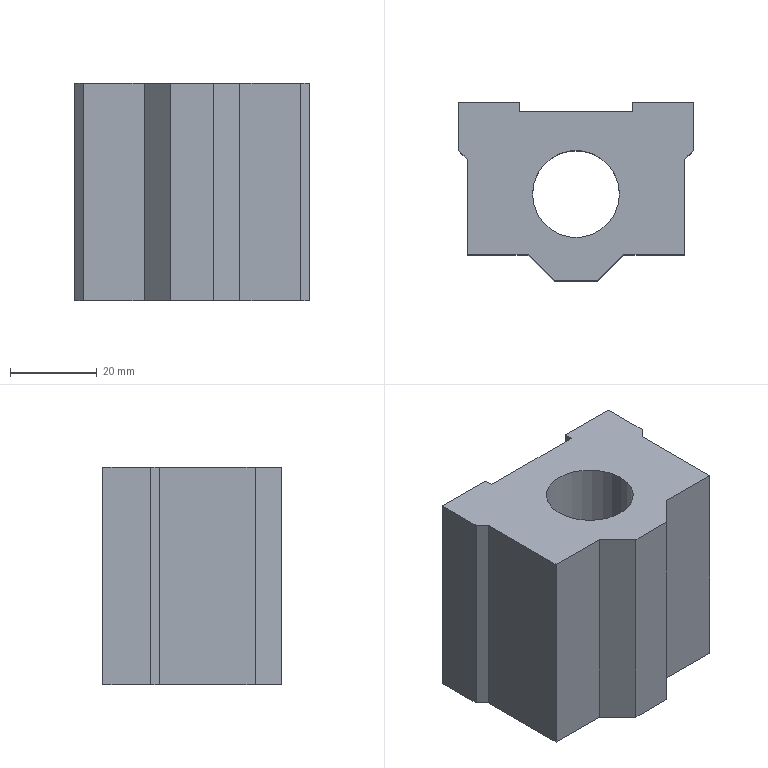Part | SolidWorks | features Extrusion 1, HoleWzd 1, LPattern 1 | 1 solid | 36 faces | box 54 x 41 x 50 mm | volume 75018 mm3 | plane 18 | cylinder 10 | cone 8 | commonest cylinder face diameters 5 x8 20 x2
STEP:
#1=CARTESIAN_POINT('',(-20.,2.498,45.));
#2=VERTEX_POINT('',#1);
#3=CARTESIAN_POINT('',(-20.,4.,47.5));
#4=VERTEX_POINT('',#3);
#5=CARTESIAN_POINT('',(-20.,4.,47.5));
#6=DIRECTION('',(0.,0.515,0.8572));
#7=VECTOR('',#6,1000.);
#8=LINE('',#5,#7);
#9=EDGE_CURVE('',#2,#4,#8,.T.);
#10=ORIENTED_EDGE('',*,*,#9,.F.);
#11=CARTESIAN_POINT('',(-20.,4.,42.5));
#12=VERTEX_POINT('',#11);
#13=CARTESIAN_POINT('',(-20.,4.,42.5));
#14=DIRECTION('',(0.,0.515,-0.8572));
#15=VECTOR('',#14,1000.);
#16=LINE('',#13,#15);
#17=EDGE_CURVE('',#2,#12,#16,.T.);
#18=ORIENTED_EDGE('',*,*,#17,.T.);
#19=CARTESIAN_POINT('',(-20.,4.,45.));
#20=DIRECTION('',(0.,1.,0.));
#21=DIRECTION('',(0.,0.,1.));
#22=AXIS2_PLACEMENT_3D('',#19,#20,#21);
#23=CIRCLE('',#22,2.5);
#24=EDGE_CURVE('',#12,#4,#23,.T.);
#25=ORIENTED_EDGE('',*,*,#24,.T.);
#26=EDGE_LOOP('',(#10,#18,#25));
#27=FACE_OUTER_BOUND('',#26,.T.);
#28=CARTESIAN_POINT('',(-20.,4.,45.));
#29=DIRECTION('',(0.,1.,0.));
#30=DIRECTION('',(0.,0.,1.));
#31=AXIS2_PLACEMENT_3D('',#28,#29,#30);
#32=CONICAL_SURFACE('',#31,2.5,1.03);
#33=ADVANCED_FACE('',(#27),#32,.F.);
#34=ORIENTED_EDGE('',*,*,#24,.F.);
#35=CARTESIAN_POINT('',(-20.,21.,42.5));
#36=VERTEX_POINT('',#35);
#37=CARTESIAN_POINT('',(-20.,21.,42.5));
#38=DIRECTION('',(0.,1.,0.));
#39=VECTOR('',#38,1000.);
#40=LINE('',#37,#39);
#41=EDGE_CURVE('',#12,#36,#40,.T.);
#42=ORIENTED_EDGE('',*,*,#41,.T.);
#43=CARTESIAN_POINT('',(-20.,21.,47.5));
#44=VERTEX_POINT('',#43);
#45=CARTESIAN_POINT('',(-20.,21.,45.));
#46=DIRECTION('',(0.,1.,0.));
#47=DIRECTION('',(0.,0.,1.));
#48=AXIS2_PLACEMENT_3D('',#45,#46,#47);
#49=CIRCLE('',#48,2.5);
#50=EDGE_CURVE('',#36,#44,#49,.T.);
#51=ORIENTED_EDGE('',*,*,#50,.T.);
#52=CARTESIAN_POINT('',(-20.,21.,47.5));
#53=DIRECTION('',(0.,1.,0.));
#54=VECTOR('',#53,1000.);
#55=LINE('',#52,#54);
#56=EDGE_CURVE('',#4,#44,#55,.T.);
#57=ORIENTED_EDGE('',*,*,#56,.F.);
#58=EDGE_LOOP('',(#34,#42,#51,#57));
#59=FACE_OUTER_BOUND('',#58,.T.);
#60=CARTESIAN_POINT('',(-20.,21.,45.));
#61=DIRECTION('',(0.,1.,0.));
#62=DIRECTION('',(0.,0.,1.));
#63=AXIS2_PLACEMENT_3D('',#60,#61,#62);
#64=CYLINDRICAL_SURFACE('',#63,2.5);
#65=ADVANCED_FACE('',(#59),#64,.F.);
#66=CARTESIAN_POINT('',(20.,2.498,45.));
#67=VERTEX_POINT('',#66);
#68=CARTESIAN_POINT('',(20.,4.,47.5));
#69=VERTEX_POINT('',#68);
#70=CARTESIAN_POINT('',(20.,4.,47.5));
#71=DIRECTION('',(0.,0.515,0.8572));
#72=VECTOR('',#71,1000.);
#73=LINE('',#70,#72);
#74=EDGE_CURVE('',#67,#69,#73,.T.);
#75=ORIENTED_EDGE('',*,*,#74,.F.);
#76=CARTESIAN_POINT('',(20.,4.,42.5));
#77=VERTEX_POINT('',#76);
#78=CARTESIAN_POINT('',(20.,4.,42.5));
#79=DIRECTION('',(0.,0.515,-0.8572));
#80=VECTOR('',#79,1000.);
#81=LINE('',#78,#80);
#82=EDGE_CURVE('',#67,#77,#81,.T.);
#83=ORIENTED_EDGE('',*,*,#82,.T.);
#84=CARTESIAN_POINT('',(20.,4.,45.));
#85=DIRECTION('',(0.,1.,0.));
#86=DIRECTION('',(0.,0.,1.));
#87=AXIS2_PLACEMENT_3D('',#84,#85,#86);
#88=CIRCLE('',#87,2.5);
#89=EDGE_CURVE('',#77,#69,#88,.T.);
#90=ORIENTED_EDGE('',*,*,#89,.T.);
#91=EDGE_LOOP('',(#75,#83,#90));
#92=FACE_OUTER_BOUND('',#91,.T.);
#93=CARTESIAN_POINT('',(20.,4.,45.));
#94=DIRECTION('',(0.,1.,0.));
#95=DIRECTION('',(0.,0.,1.));
#96=AXIS2_PLACEMENT_3D('',#93,#94,#95);
#97=CONICAL_SURFACE('',#96,2.5,1.03);
#98=ADVANCED_FACE('',(#92),#97,.F.);
#99=ORIENTED_EDGE('',*,*,#89,.F.);
#100=CARTESIAN_POINT('',(20.,21.,42.5));
#101=VERTEX_POINT('',#100);
#102=CARTESIAN_POINT('',(20.,21.,42.5));
#103=DIRECTION('',(0.,1.,0.));
#104=VECTOR('',#103,1000.);
#105=LINE('',#102,#104);
#106=EDGE_CURVE('',#77,#101,#105,.T.);
#107=ORIENTED_EDGE('',*,*,#106,.T.);
#108=CARTESIAN_POINT('',(20.,21.,47.5));
#109=VERTEX_POINT('',#108);
#110=CARTESIAN_POINT('',(20.,21.,45.));
#111=DIRECTION('',(0.,1.,0.));
#112=DIRECTION('',(0.,0.,1.));
#113=AXIS2_PLACEMENT_3D('',#110,#111,#112);
#114=CIRCLE('',#113,2.5);
#115=EDGE_CURVE('',#101,#109,#114,.T.);
#116=ORIENTED_EDGE('',*,*,#115,.T.);
#117=CARTESIAN_POINT('',(20.,21.,47.5));
#118=DIRECTION('',(0.,1.,0.));
#119=VECTOR('',#118,1000.);
#120=LINE('',#117,#119);
#121=EDGE_CURVE('',#69,#109,#120,.T.);
#122=ORIENTED_EDGE('',*,*,#121,.F.);
#123=EDGE_LOOP('',(#99,#107,#116,#122));
#124=FACE_OUTER_BOUND('',#123,.T.);
#125=CARTESIAN_POINT('',(20.,21.,45.));
#126=DIRECTION('',(0.,1.,0.));
#127=DIRECTION('',(0.,0.,1.));
#128=AXIS2_PLACEMENT_3D('',#125,#126,#127);
#129=CYLINDRICAL_SURFACE('',#128,2.5);
#130=ADVANCED_FACE('',(#124),#129,.F.);
#131=CARTESIAN_POINT('',(-20.,2.498,5.));
#132=VERTEX_POINT('',#131);
#133=CARTESIAN_POINT('',(-20.,4.,7.5));
#134=VERTEX_POINT('',#133);
#135=CARTESIAN_POINT('',(-20.,4.,7.5));
#136=DIRECTION('',(0.,0.515,0.8572));
#137=VECTOR('',#136,1000.);
#138=LINE('',#135,#137);
#139=EDGE_CURVE('',#132,#134,#138,.T.);
#140=ORIENTED_EDGE('',*,*,#139,.F.);
#141=CARTESIAN_POINT('',(-20.,4.,2.5));
#142=VERTEX_POINT('',#141);
#143=CARTESIAN_POINT('',(-20.,4.,2.5));
#144=DIRECTION('',(0.,0.515,-0.8572));
#145=VECTOR('',#144,1000.);
#146=LINE('',#143,#145);
#147=EDGE_CURVE('',#132,#142,#146,.T.);
#148=ORIENTED_EDGE('',*,*,#147,.T.);
#149=CARTESIAN_POINT('',(-20.,4.,5.));
#150=DIRECTION('',(0.,1.,0.));
#151=DIRECTION('',(0.,0.,1.));
#152=AXIS2_PLACEMENT_3D('',#149,#150,#151);
#153=CIRCLE('',#152,2.5);
#154=EDGE_CURVE('',#142,#134,#153,.T.);
#155=ORIENTED_EDGE('',*,*,#154,.T.);
#156=EDGE_LOOP('',(#140,#148,#155));
#157=FACE_OUTER_BOUND('',#156,.T.);
#158=CARTESIAN_POINT('',(-20.,4.,5.));
#159=DIRECTION('',(0.,1.,0.));
#160=DIRECTION('',(0.,0.,1.));
#161=AXIS2_PLACEMENT_3D('',#158,#159,#160);
#162=CONICAL_SURFACE('',#161,2.5,1.03);
#163=ADVANCED_FACE('',(#157),#162,.F.);
#164=ORIENTED_EDGE('',*,*,#154,.F.);
#165=CARTESIAN_POINT('',(-20.,21.,2.5));
#166=VERTEX_POINT('',#165);
#167=CARTESIAN_POINT('',(-20.,21.,2.5));
#168=DIRECTION('',(0.,1.,0.));
#169=VECTOR('',#168,1000.);
#170=LINE('',#167,#169);
#171=EDGE_CURVE('',#142,#166,#170,.T.);
#172=ORIENTED_EDGE('',*,*,#171,.T.);
#173=CARTESIAN_POINT('',(-20.,21.,7.5));
#174=VERTEX_POINT('',#173);
#175=CARTESIAN_POINT('',(-20.,21.,5.));
#176=DIRECTION('',(0.,1.,0.));
#177=DIRECTION('',(0.,0.,1.));
#178=AXIS2_PLACEMENT_3D('',#175,#176,#177);
#179=CIRCLE('',#178,2.5);
#180=EDGE_CURVE('',#166,#174,#179,.T.);
#181=ORIENTED_EDGE('',*,*,#180,.T.);
#182=CARTESIAN_POINT('',(-20.,21.,7.5));
#183=DIRECTION('',(0.,1.,0.));
#184=VECTOR('',#183,1000.);
#185=LINE('',#182,#184);
#186=EDGE_CURVE('',#134,#174,#185,.T.);
#187=ORIENTED_EDGE('',*,*,#186,.F.);
#188=EDGE_LOOP('',(#164,#172,#181,#187));
#189=FACE_OUTER_BOUND('',#188,.T.);
#190=CARTESIAN_POINT('',(-20.,21.,5.));
#191=DIRECTION('',(0.,1.,0.));
#192=DIRECTION('',(0.,0.,1.));
#193=AXIS2_PLACEMENT_3D('',#190,#191,#192);
#194=CYLINDRICAL_SURFACE('',#193,2.5);
#195=ADVANCED_FACE('',(#189),#194,.F.);
#196=CARTESIAN_POINT('',(20.,2.498,5.));
#197=VERTEX_POINT('',#196);
#198=CARTESIAN_POINT('',(20.,4.,7.5));
#199=VERTEX_POINT('',#198);
#200=CARTESIAN_POINT('',(20.,4.,7.5));
#201=DIRECTION('',(0.,0.515,0.8572));
#202=VECTOR('',#201,1000.);
#203=LINE('',#200,#202);
#204=EDGE_CURVE('',#197,#199,#203,.T.);
#205=ORIENTED_EDGE('',*,*,#204,.F.);
#206=CARTESIAN_POINT('',(20.,4.,2.5));
#207=VERTEX_POINT('',#206);
#208=CARTESIAN_POINT('',(20.,4.,2.5));
#209=DIRECTION('',(0.,0.515,-0.8572));
#210=VECTOR('',#209,1000.);
#211=LINE('',#208,#210);
#212=EDGE_CURVE('',#197,#207,#211,.T.);
#213=ORIENTED_EDGE('',*,*,#212,.T.);
#214=CARTESIAN_POINT('',(20.,4.,5.));
#215=DIRECTION('',(0.,1.,0.));
#216=DIRECTION('',(0.,0.,1.));
#217=AXIS2_PLACEMENT_3D('',#214,#215,#216);
#218=CIRCLE('',#217,2.5);
#219=EDGE_CURVE('',#207,#199,#218,.T.);
#220=ORIENTED_EDGE('',*,*,#219,.T.);
#221=EDGE_LOOP('',(#205,#213,#220));
#222=FACE_OUTER_BOUND('',#221,.T.);
#223=CARTESIAN_POINT('',(20.,4.,5.));
#224=DIRECTION('',(0.,1.,0.));
#225=DIRECTION('',(0.,0.,1.));
#226=AXIS2_PLACEMENT_3D('',#223,#224,#225);
#227=CONICAL_SURFACE('',#226,2.5,1.03);
#228=ADVANCED_FACE('',(#222),#227,.F.);
#229=ORIENTED_EDGE('',*,*,#219,.F.);
#230=CARTESIAN_POINT('',(20.,21.,2.5));
#231=VERTEX_POINT('',#230);
#232=CARTESIAN_POINT('',(20.,21.,2.5));
#233=DIRECTION('',(0.,1.,0.));
#234=VECTOR('',#233,1000.);
#235=LINE('',#232,#234);
#236=EDGE_CURVE('',#207,#231,#235,.T.);
#237=ORIENTED_EDGE('',*,*,#236,.T.);
#238=CARTESIAN_POINT('',(20.,21.,7.5));
#239=VERTEX_POINT('',#238);
#240=CARTESIAN_POINT('',(20.,21.,5.));
#241=DIRECTION('',(0.,1.,0.));
#242=DIRECTION('',(0.,0.,1.));
#243=AXIS2_PLACEMENT_3D('',#240,#241,#242);
#244=CIRCLE('',#243,2.5);
#245=EDGE_CURVE('',#231,#239,#244,.T.);
#246=ORIENTED_EDGE('',*,*,#245,.T.);
#247=CARTESIAN_POINT('',(20.,21.,7.5));
#248=DIRECTION('',(0.,1.,0.));
#249=VECTOR('',#248,1000.);
#250=LINE('',#247,#249);
#251=EDGE_CURVE('',#199,#239,#250,.T.);
#252=ORIENTED_EDGE('',*,*,#251,.F.);
#253=EDGE_LOOP('',(#229,#237,#246,#252));
#254=FACE_OUTER_BOUND('',#253,.T.);
#255=CARTESIAN_POINT('',(20.,21.,5.));
#256=DIRECTION('',(0.,1.,0.));
#257=DIRECTION('',(0.,0.,1.));
#258=AXIS2_PLACEMENT_3D('',#255,#256,#257);
#259=CYLINDRICAL_SURFACE('',#258,2.5);
#260=ADVANCED_FACE('',(#254),#259,.F.);
#261=CARTESIAN_POINT('',(-10.,0.,50.));
#262=VERTEX_POINT('',#261);
#263=CARTESIAN_POINT('',(10.,0.,50.));
#264=VERTEX_POINT('',#263);
#265=CARTESIAN_POINT('',(0.,0.,50.));
#266=DIRECTION('',(0.,0.,1.));
#267=DIRECTION('',(1.,0.,0.));
#268=AXIS2_PLACEMENT_3D('',#265,#266,#267);
#269=CIRCLE('',#268,10.);
#270=EDGE_CURVE('',#262,#264,#269,.T.);
#271=ORIENTED_EDGE('',*,*,#270,.T.);
#272=CARTESIAN_POINT('',(10.,0.,0.));
#273=VERTEX_POINT('',#272);
#274=CARTESIAN_POINT('',(10.,0.,50.));
#275=DIRECTION('',(0.,0.,-1.));
#276=VECTOR('',#275,1000.);
#277=LINE('',#274,#276);
#278=EDGE_CURVE('',#264,#273,#277,.T.);
#279=ORIENTED_EDGE('',*,*,#278,.T.);
#280=CARTESIAN_POINT('',(-10.,0.,0.));
#281=VERTEX_POINT('',#280);
#282=CARTESIAN_POINT('',(0.,0.,0.));
#283=DIRECTION('',(0.,0.,1.));
#284=DIRECTION('',(1.,0.,0.));
#285=AXIS2_PLACEMENT_3D('',#282,#283,#284);
#286=CIRCLE('',#285,10.);
#287=EDGE_CURVE('',#281,#273,#286,.T.);
#288=ORIENTED_EDGE('',*,*,#287,.F.);
#289=CARTESIAN_POINT('',(-10.,0.,50.));
#290=DIRECTION('',(0.,0.,-1.));
#291=VECTOR('',#290,1000.);
#292=LINE('',#289,#291);
#293=EDGE_CURVE('',#262,#281,#292,.T.);
#294=ORIENTED_EDGE('',*,*,#293,.F.);
#295=EDGE_LOOP('',(#271,#279,#288,#294));
#296=FACE_OUTER_BOUND('',#295,.T.);
#297=CARTESIAN_POINT('',(0.,0.,50.));
#298=DIRECTION('',(0.,0.,-1.));
#299=DIRECTION('',(-1.,0.,0.));
#300=AXIS2_PLACEMENT_3D('',#297,#298,#299);
#301=CYLINDRICAL_SURFACE('',#300,10.);
#302=ADVANCED_FACE('',(#296),#301,.F.);
#303=CARTESIAN_POINT('',(-11.,-14.,50.));
#304=VERTEX_POINT('',#303);
#305=CARTESIAN_POINT('',(-5.,-20.,50.));
#306=VERTEX_POINT('',#305);
#307=CARTESIAN_POINT('',(-5.,-20.,50.));
#308=DIRECTION('',(0.7071,-0.7071,0.));
#309=VECTOR('',#308,1000.);
#310=LINE('',#307,#309);
#311=EDGE_CURVE('',#304,#306,#310,.T.);
#312=ORIENTED_EDGE('',*,*,#311,.T.);
#313=CARTESIAN_POINT('',(5.,-20.,50.));
#314=VERTEX_POINT('',#313);
#315=CARTESIAN_POINT('',(5.,-20.,50.));
#316=DIRECTION('',(1.,0.,0.));
#317=VECTOR('',#316,1000.);
#318=LINE('',#315,#317);
#319=EDGE_CURVE('',#306,#314,#318,.T.);
#320=ORIENTED_EDGE('',*,*,#319,.T.);
#321=CARTESIAN_POINT('',(11.,-14.,50.));
#322=VERTEX_POINT('',#321);
#323=CARTESIAN_POINT('',(5.,-20.,50.));
#324=DIRECTION('',(0.7071,0.7071,0.));
#325=VECTOR('',#324,1000.);
#326=LINE('',#323,#325);
#327=EDGE_CURVE('',#314,#322,#326,.T.);
#328=ORIENTED_EDGE('',*,*,#327,.T.);
#329=CARTESIAN_POINT('',(25.,-14.,50.));
#330=VERTEX_POINT('',#329);
#331=CARTESIAN_POINT('',(11.,-14.,50.));
#332=DIRECTION('',(1.,0.,0.));
#333=VECTOR('',#332,1000.);
#334=LINE('',#331,#333);
#335=EDGE_CURVE('',#322,#330,#334,.T.);
#336=ORIENTED_EDGE('',*,*,#335,.T.);
#337=CARTESIAN_POINT('',(25.,8.,50.));
#338=VERTEX_POINT('',#337);
#339=CARTESIAN_POINT('',(25.,-14.,50.));
#340=DIRECTION('',(0.,1.,0.));
#341=VECTOR('',#340,1000.);
#342=LINE('',#339,#341);
#343=EDGE_CURVE('',#330,#338,#342,.T.);
#344=ORIENTED_EDGE('',*,*,#343,.T.);
#345=CARTESIAN_POINT('',(27.,10.,50.));
#346=VERTEX_POINT('',#345);
#347=CARTESIAN_POINT('',(25.,8.,50.));
#348=DIRECTION('',(0.7071,0.7071,0.));
#349=VECTOR('',#348,1000.);
#350=LINE('',#347,#349);
#351=EDGE_CURVE('',#338,#346,#350,.T.);
#352=ORIENTED_EDGE('',*,*,#351,.T.);
#353=CARTESIAN_POINT('',(27.,21.,50.));
#354=VERTEX_POINT('',#353);
#355=CARTESIAN_POINT('',(27.,10.,50.));
#356=DIRECTION('',(0.,1.,0.));
#357=VECTOR('',#356,1000.);
#358=LINE('',#355,#357);
#359=EDGE_CURVE('',#346,#354,#358,.T.);
#360=ORIENTED_EDGE('',*,*,#359,.T.);
#361=CARTESIAN_POINT('',(13.,21.,50.));
#362=VERTEX_POINT('',#361);
#363=CARTESIAN_POINT('',(27.,21.,50.));
#364=DIRECTION('',(-1.,0.,0.));
#365=VECTOR('',#364,1000.);
#366=LINE('',#363,#365);
#367=EDGE_CURVE('',#354,#362,#366,.T.);
#368=ORIENTED_EDGE('',*,*,#367,.T.);
#369=CARTESIAN_POINT('',(13.,19.,50.));
#370=VERTEX_POINT('',#369);
#371=CARTESIAN_POINT('',(13.,21.,50.));
#372=DIRECTION('',(0.,-1.,0.));
#373=VECTOR('',#372,1000.);
#374=LINE('',#371,#373);
#375=EDGE_CURVE('',#362,#370,#374,.T.);
#376=ORIENTED_EDGE('',*,*,#375,.T.);
#377=CARTESIAN_POINT('',(-13.,19.,50.));
#378=VERTEX_POINT('',#377);
#379=CARTESIAN_POINT('',(-13.,19.,50.));
#380=DIRECTION('',(-1.,0.,0.));
#381=VECTOR('',#380,1000.);
#382=LINE('',#379,#381);
#383=EDGE_CURVE('',#370,#378,#382,.T.);
#384=ORIENTED_EDGE('',*,*,#383,.T.);
#385=CARTESIAN_POINT('',(-13.,21.,50.));
#386=VERTEX_POINT('',#385);
#387=CARTESIAN_POINT('',(-13.,21.,50.));
#388=DIRECTION('',(0.,1.,0.));
#389=VECTOR('',#388,1000.);
#390=LINE('',#387,#389);
#391=EDGE_CURVE('',#378,#386,#390,.T.);
#392=ORIENTED_EDGE('',*,*,#391,.T.);
#393=CARTESIAN_POINT('',(-27.,21.,50.));
#394=VERTEX_POINT('',#393);
#395=CARTESIAN_POINT('',(-27.,21.,50.));
#396=DIRECTION('',(-1.,0.,0.));
#397=VECTOR('',#396,1000.);
#398=LINE('',#395,#397);
#399=EDGE_CURVE('',#386,#394,#398,.T.);
#400=ORIENTED_EDGE('',*,*,#399,.T.);
#401=CARTESIAN_POINT('',(-27.,10.,50.));
#402=VERTEX_POINT('',#401);
#403=CARTESIAN_POINT('',(-27.,10.,50.));
#404=DIRECTION('',(0.,-1.,0.));
#405=VECTOR('',#404,1000.);
#406=LINE('',#403,#405);
#407=EDGE_CURVE('',#394,#402,#406,.T.);
#408=ORIENTED_EDGE('',*,*,#407,.T.);
#409=CARTESIAN_POINT('',(-25.,8.,50.));
#410=VERTEX_POINT('',#409);
#411=CARTESIAN_POINT('',(-25.,8.,50.));
#412=DIRECTION('',(0.7071,-0.7071,0.));
#413=VECTOR('',#412,1000.);
#414=LINE('',#411,#413);
#415=EDGE_CURVE('',#402,#410,#414,.T.);
#416=ORIENTED_EDGE('',*,*,#415,.T.);
#417=CARTESIAN_POINT('',(-25.,-14.,50.));
#418=VERTEX_POINT('',#417);
#419=CARTESIAN_POINT('',(-25.,-14.,50.));
#420=DIRECTION('',(0.,-1.,0.));
#421=VECTOR('',#420,1000.);
#422=LINE('',#419,#421);
#423=EDGE_CURVE('',#410,#418,#422,.T.);
#424=ORIENTED_EDGE('',*,*,#423,.T.);
#425=CARTESIAN_POINT('',(-11.,-14.,50.));
#426=DIRECTION('',(1.,0.,0.));
#427=VECTOR('',#426,1000.);
#428=LINE('',#425,#427);
#429=EDGE_CURVE('',#418,#304,#428,.T.);
#430=ORIENTED_EDGE('',*,*,#429,.T.);
#431=EDGE_LOOP('',(#312,#320,#328,#336,#344,#352,#360,#368,#376,#384,#392,#400,#408,#416,#424,#430));
#432=FACE_OUTER_BOUND('',#431,.T.);
#433=ORIENTED_EDGE('',*,*,#270,.F.);
#434=CARTESIAN_POINT('',(0.,0.,50.));
#435=DIRECTION('',(0.,0.,1.));
#436=DIRECTION('',(1.,0.,0.));
#437=AXIS2_PLACEMENT_3D('',#434,#435,#436);
#438=CIRCLE('',#437,10.);
#439=EDGE_CURVE('',#264,#262,#438,.T.);
#440=ORIENTED_EDGE('',*,*,#439,.F.);
#441=EDGE_LOOP('',(#433,#440));
#442=FACE_BOUND('',#441,.T.);
#443=CARTESIAN_POINT('',(-4.,-21.,50.));
#444=DIRECTION('',(0.,0.,-1.));
#445=DIRECTION('',(-1.,0.,0.));
#446=AXIS2_PLACEMENT_3D('',#443,#444,#445);
#447=PLANE('',#446);
#448=ADVANCED_FACE('',(#432,#442),#447,.F.);
#449=CARTESIAN_POINT('',(-11.,-14.,0.));
#450=VERTEX_POINT('',#449);
#451=CARTESIAN_POINT('',(-5.,-20.,0.));
#452=VERTEX_POINT('',#451);
#453=CARTESIAN_POINT('',(-5.,-20.,0.));
#454=DIRECTION('',(0.7071,-0.7071,0.));
#455=VECTOR('',#454,1000.);
#456=LINE('',#453,#455);
#457=EDGE_CURVE('',#450,#452,#456,.T.);
#458=ORIENTED_EDGE('',*,*,#457,.F.);
#459=CARTESIAN_POINT('',(-25.,-14.,0.));
#460=VERTEX_POINT('',#459);
#461=CARTESIAN_POINT('',(-11.,-14.,0.));
#462=DIRECTION('',(1.,0.,0.));
#463=VECTOR('',#462,1000.);
#464=LINE('',#461,#463);
#465=EDGE_CURVE('',#460,#450,#464,.T.);
#466=ORIENTED_EDGE('',*,*,#465,.F.);
#467=CARTESIAN_POINT('',(-25.,8.,0.));
#468=VERTEX_POINT('',#467);
#469=CARTESIAN_POINT('',(-25.,-14.,0.));
#470=DIRECTION('',(0.,-1.,0.));
#471=VECTOR('',#470,1000.);
#472=LINE('',#469,#471);
#473=EDGE_CURVE('',#468,#460,#472,.T.);
#474=ORIENTED_EDGE('',*,*,#473,.F.);
#475=CARTESIAN_POINT('',(-27.,10.,0.));
#476=VERTEX_POINT('',#475);
#477=CARTESIAN_POINT('',(-25.,8.,0.));
#478=DIRECTION('',(0.7071,-0.7071,0.));
#479=VECTOR('',#478,1000.);
#480=LINE('',#477,#479);
#481=EDGE_CURVE('',#476,#468,#480,.T.);
#482=ORIENTED_EDGE('',*,*,#481,.F.);
#483=CARTESIAN_POINT('',(-27.,21.,0.));
#484=VERTEX_POINT('',#483);
#485=CARTESIAN_POINT('',(-27.,10.,0.));
#486=DIRECTION('',(0.,-1.,0.));
#487=VECTOR('',#486,1000.);
#488=LINE('',#485,#487);
#489=EDGE_CURVE('',#484,#476,#488,.T.);
#490=ORIENTED_EDGE('',*,*,#489,.F.);
#491=CARTESIAN_POINT('',(-13.,21.,0.));
#492=VERTEX_POINT('',#491);
#493=CARTESIAN_POINT('',(-27.,21.,0.));
#494=DIRECTION('',(-1.,0.,0.));
#495=VECTOR('',#494,1000.);
#496=LINE('',#493,#495);
#497=EDGE_CURVE('',#492,#484,#496,.T.);
#498=ORIENTED_EDGE('',*,*,#497,.F.);
#499=CARTESIAN_POINT('',(-13.,19.,0.));
#500=VERTEX_POINT('',#499);
#501=CARTESIAN_POINT('',(-13.,21.,0.));
#502=DIRECTION('',(0.,1.,0.));
#503=VECTOR('',#502,1000.);
#504=LINE('',#501,#503);
#505=EDGE_CURVE('',#500,#492,#504,.T.);
#506=ORIENTED_EDGE('',*,*,#505,.F.);
#507=CARTESIAN_POINT('',(13.,19.,0.));
#508=VERTEX_POINT('',#507);
#509=CARTESIAN_POINT('',(-13.,19.,0.));
#510=DIRECTION('',(-1.,0.,0.));
#511=VECTOR('',#510,1000.);
#512=LINE('',#509,#511);
#513=EDGE_CURVE('',#508,#500,#512,.T.);
#514=ORIENTED_EDGE('',*,*,#513,.F.);
#515=CARTESIAN_POINT('',(13.,21.,0.));
#516=VERTEX_POINT('',#515);
#517=CARTESIAN_POINT('',(13.,21.,0.));
#518=DIRECTION('',(0.,-1.,0.));
#519=VECTOR('',#518,1000.);
#520=LINE('',#517,#519);
#521=EDGE_CURVE('',#516,#508,#520,.T.);
#522=ORIENTED_EDGE('',*,*,#521,.F.);
#523=CARTESIAN_POINT('',(27.,21.,0.));
#524=VERTEX_POINT('',#523);
#525=CARTESIAN_POINT('',(27.,21.,0.));
#526=DIRECTION('',(-1.,0.,0.));
#527=VECTOR('',#526,1000.);
#528=LINE('',#525,#527);
#529=EDGE_CURVE('',#524,#516,#528,.T.);
#530=ORIENTED_EDGE('',*,*,#529,.F.);
#531=CARTESIAN_POINT('',(27.,10.,0.));
#532=VERTEX_POINT('',#531);
#533=CARTESIAN_POINT('',(27.,10.,0.));
#534=DIRECTION('',(0.,1.,0.));
#535=VECTOR('',#534,1000.);
#536=LINE('',#533,#535);
#537=EDGE_CURVE('',#532,#524,#536,.T.);
#538=ORIENTED_EDGE('',*,*,#537,.F.);
#539=CARTESIAN_POINT('',(25.,8.,0.));
#540=VERTEX_POINT('',#539);
#541=CARTESIAN_POINT('',(25.,8.,0.));
#542=DIRECTION('',(0.7071,0.7071,0.));
#543=VECTOR('',#542,1000.);
#544=LINE('',#541,#543);
#545=EDGE_CURVE('',#540,#532,#544,.T.);
#546=ORIENTED_EDGE('',*,*,#545,.F.);
#547=CARTESIAN_POINT('',(25.,-14.,0.));
#548=VERTEX_POINT('',#547);
#549=CARTESIAN_POINT('',(25.,-14.,0.));
#550=DIRECTION('',(0.,1.,0.));
#551=VECTOR('',#550,1000.);
#552=LINE('',#549,#551);
#553=EDGE_CURVE('',#548,#540,#552,.T.);
#554=ORIENTED_EDGE('',*,*,#553,.F.);
#555=CARTESIAN_POINT('',(11.,-14.,0.));
#556=VERTEX_POINT('',#555);
#557=CARTESIAN_POINT('',(11.,-14.,0.));
#558=DIRECTION('',(1.,0.,0.));
#559=VECTOR('',#558,1000.);
#560=LINE('',#557,#559);
#561=EDGE_CURVE('',#556,#548,#560,.T.);
#562=ORIENTED_EDGE('',*,*,#561,.F.);
#563=CARTESIAN_POINT('',(5.,-20.,0.));
#564=VERTEX_POINT('',#563);
#565=CARTESIAN_POINT('',(5.,-20.,0.));
#566=DIRECTION('',(0.7071,0.7071,0.));
#567=VECTOR('',#566,1000.);
#568=LINE('',#565,#567);
#569=EDGE_CURVE('',#564,#556,#568,.T.);
#570=ORIENTED_EDGE('',*,*,#569,.F.);
#571=CARTESIAN_POINT('',(5.,-20.,0.));
#572=DIRECTION('',(1.,0.,0.));
#573=VECTOR('',#572,1000.);
#574=LINE('',#571,#573);
#575=EDGE_CURVE('',#452,#564,#574,.T.);
#576=ORIENTED_EDGE('',*,*,#575,.F.);
#577=EDGE_LOOP('',(#458,#466,#474,#482,#490,#498,#506,#514,#522,#530,#538,#546,#554,#562,#570,#576));
#578=FACE_OUTER_BOUND('',#577,.T.);
#579=ORIENTED_EDGE('',*,*,#287,.T.);
#580=CARTESIAN_POINT('',(0.,0.,0.));
#581=DIRECTION('',(0.,0.,1.));
#582=DIRECTION('',(1.,0.,0.));
#583=AXIS2_PLACEMENT_3D('',#580,#581,#582);
#584=CIRCLE('',#583,10.);
#585=EDGE_CURVE('',#273,#281,#584,.T.);
#586=ORIENTED_EDGE('',*,*,#585,.T.);
#587=EDGE_LOOP('',(#579,#586));
#588=FACE_BOUND('',#587,.T.);
#589=CARTESIAN_POINT('',(-4.,-21.,0.));
#590=DIRECTION('',(0.,0.,-1.));
#591=DIRECTION('',(-1.,0.,0.));
#592=AXIS2_PLACEMENT_3D('',#589,#590,#591);
#593=PLANE('',#592);
#594=ADVANCED_FACE('',(#578,#588),#593,.T.);
#595=ORIENTED_EDGE('',*,*,#457,.T.);
#596=CARTESIAN_POINT('',(-5.,-20.,50.));
#597=DIRECTION('',(0.,0.,-1.));
#598=VECTOR('',#597,1000.);
#599=LINE('',#596,#598);
#600=EDGE_CURVE('',#306,#452,#599,.T.);
#601=ORIENTED_EDGE('',*,*,#600,.F.);
#602=ORIENTED_EDGE('',*,*,#311,.F.);
#603=CARTESIAN_POINT('',(-11.,-14.,50.));
#604=DIRECTION('',(0.,0.,-1.));
#605=VECTOR('',#604,1000.);
#606=LINE('',#603,#605);
#607=EDGE_CURVE('',#304,#450,#606,.T.);
#608=ORIENTED_EDGE('',*,*,#607,.T.);
#609=EDGE_LOOP('',(#595,#601,#602,#608));
#610=FACE_OUTER_BOUND('',#609,.T.);
#611=CARTESIAN_POINT('',(-5.,-20.,50.));
#612=DIRECTION('',(0.7071,0.7071,0.));
#613=DIRECTION('',(-0.7071,0.7071,0.));
#614=AXIS2_PLACEMENT_3D('',#611,#612,#613);
#615=PLANE('',#614);
#616=ADVANCED_FACE('',(#610),#615,.F.);
#617=ORIENTED_EDGE('',*,*,#575,.T.);
#618=CARTESIAN_POINT('',(5.,-20.,50.));
#619=DIRECTION('',(0.,0.,-1.));
#620=VECTOR('',#619,1000.);
#621=LINE('',#618,#620);
#622=EDGE_CURVE('',#314,#564,#621,.T.);
#623=ORIENTED_EDGE('',*,*,#622,.F.);
#624=ORIENTED_EDGE('',*,*,#319,.F.);
#625=ORIENTED_EDGE('',*,*,#600,.T.);
#626=EDGE_LOOP('',(#617,#623,#624,#625));
#627=FACE_OUTER_BOUND('',#626,.T.);
#628=CARTESIAN_POINT('',(5.,-20.,50.));
#629=DIRECTION('',(0.,1.,0.));
#630=DIRECTION('',(0.,0.,1.));
#631=AXIS2_PLACEMENT_3D('',#628,#629,#630);
#632=PLANE('',#631);
#633=ADVANCED_FACE('',(#627),#632,.F.);
#634=ORIENTED_EDGE('',*,*,#569,.T.);
#635=CARTESIAN_POINT('',(11.,-14.,50.));
#636=DIRECTION('',(0.,0.,-1.));
#637=VECTOR('',#636,1000.);
#638=LINE('',#635,#637);
#639=EDGE_CURVE('',#322,#556,#638,.T.);
#640=ORIENTED_EDGE('',*,*,#639,.F.);
#641=ORIENTED_EDGE('',*,*,#327,.F.);
#642=ORIENTED_EDGE('',*,*,#622,.T.);
#643=EDGE_LOOP('',(#634,#640,#641,#642));
#644=FACE_OUTER_BOUND('',#643,.T.);
#645=CARTESIAN_POINT('',(5.,-20.,50.));
#646=DIRECTION('',(-0.7071,0.7071,0.));
#647=DIRECTION('',(-0.7071,-0.7071,0.));
#648=AXIS2_PLACEMENT_3D('',#645,#646,#647);
#649=PLANE('',#648);
#650=ADVANCED_FACE('',(#644),#649,.F.);
#651=ORIENTED_EDGE('',*,*,#561,.T.);
#652=CARTESIAN_POINT('',(25.,-14.,50.));
#653=DIRECTION('',(0.,0.,-1.));
#654=VECTOR('',#653,1000.);
#655=LINE('',#652,#654);
#656=EDGE_CURVE('',#330,#548,#655,.T.);
#657=ORIENTED_EDGE('',*,*,#656,.F.);
#658=ORIENTED_EDGE('',*,*,#335,.F.);
#659=ORIENTED_EDGE('',*,*,#639,.T.);
#660=EDGE_LOOP('',(#651,#657,#658,#659));
#661=FACE_OUTER_BOUND('',#660,.T.);
#662=CARTESIAN_POINT('',(11.,-14.,50.));
#663=DIRECTION('',(0.,1.,0.));
#664=DIRECTION('',(-1.,0.,0.));
#665=AXIS2_PLACEMENT_3D('',#662,#663,#664);
#666=PLANE('',#665);
#667=ADVANCED_FACE('',(#661),#666,.F.);
#668=ORIENTED_EDGE('',*,*,#553,.T.);
#669=CARTESIAN_POINT('',(25.,8.,50.));
#670=DIRECTION('',(0.,0.,-1.));
#671=VECTOR('',#670,1000.);
#672=LINE('',#669,#671);
#673=EDGE_CURVE('',#338,#540,#672,.T.);
#674=ORIENTED_EDGE('',*,*,#673,.F.);
#675=ORIENTED_EDGE('',*,*,#343,.F.);
#676=ORIENTED_EDGE('',*,*,#656,.T.);
#677=EDGE_LOOP('',(#668,#674,#675,#676));
#678=FACE_OUTER_BOUND('',#677,.T.);
#679=CARTESIAN_POINT('',(25.,-14.,50.));
#680=DIRECTION('',(-1.,0.,0.));
#681=DIRECTION('',(0.,-1.,0.));
#682=AXIS2_PLACEMENT_3D('',#679,#680,#681);
#683=PLANE('',#682);
#684=ADVANCED_FACE('',(#678),#683,.F.);
#685=ORIENTED_EDGE('',*,*,#545,.T.);
#686=CARTESIAN_POINT('',(27.,10.,50.));
#687=DIRECTION('',(0.,0.,-1.));
#688=VECTOR('',#687,1000.);
#689=LINE('',#686,#688);
#690=EDGE_CURVE('',#346,#532,#689,.T.);
#691=ORIENTED_EDGE('',*,*,#690,.F.);
#692=ORIENTED_EDGE('',*,*,#351,.F.);
#693=ORIENTED_EDGE('',*,*,#673,.T.);
#694=EDGE_LOOP('',(#685,#691,#692,#693));
#695=FACE_OUTER_BOUND('',#694,.T.);
#696=CARTESIAN_POINT('',(25.,8.,50.));
#697=DIRECTION('',(-0.7071,0.7071,0.));
#698=DIRECTION('',(-0.7071,-0.7071,0.));
#699=AXIS2_PLACEMENT_3D('',#696,#697,#698);
#700=PLANE('',#699);
#701=ADVANCED_FACE('',(#695),#700,.F.);
#702=ORIENTED_EDGE('',*,*,#537,.T.);
#703=CARTESIAN_POINT('',(27.,21.,50.));
#704=DIRECTION('',(0.,0.,-1.));
#705=VECTOR('',#704,1000.);
#706=LINE('',#703,#705);
#707=EDGE_CURVE('',#354,#524,#706,.T.);
#708=ORIENTED_EDGE('',*,*,#707,.F.);
#709=ORIENTED_EDGE('',*,*,#359,.F.);
#710=ORIENTED_EDGE('',*,*,#690,.T.);
#711=EDGE_LOOP('',(#702,#708,#709,#710));
#712=FACE_OUTER_BOUND('',#711,.T.);
#713=CARTESIAN_POINT('',(27.,10.,50.));
#714=DIRECTION('',(-1.,0.,0.));
#715=DIRECTION('',(0.,0.,1.));
#716=AXIS2_PLACEMENT_3D('',#713,#714,#715);
#717=PLANE('',#716);
#718=ADVANCED_FACE('',(#712),#717,.F.);
#719=CARTESIAN_POINT('',(20.,21.,45.));
#720=DIRECTION('',(0.,1.,0.));
#721=DIRECTION('',(0.,0.,1.));
#722=AXIS2_PLACEMENT_3D('',#719,#720,#721);
#723=CIRCLE('',#722,2.5);
#724=EDGE_CURVE('',#109,#101,#723,.T.);
#725=ORIENTED_EDGE('',*,*,#724,.F.);
#726=ORIENTED_EDGE('',*,*,#115,.F.);
#727=EDGE_LOOP('',(#725,#726));
#728=FACE_BOUND('',#727,.T.);
#729=CARTESIAN_POINT('',(20.,21.,5.));
#730=DIRECTION('',(0.,1.,0.));
#731=DIRECTION('',(0.,0.,1.));
#732=AXIS2_PLACEMENT_3D('',#729,#730,#731);
#733=CIRCLE('',#732,2.5);
#734=EDGE_CURVE('',#239,#231,#733,.T.);
#735=ORIENTED_EDGE('',*,*,#734,.F.);
#736=ORIENTED_EDGE('',*,*,#245,.F.);
#737=EDGE_LOOP('',(#735,#736));
#738=FACE_BOUND('',#737,.T.);
#739=ORIENTED_EDGE('',*,*,#529,.T.);
#740=CARTESIAN_POINT('',(13.,21.,50.));
#741=DIRECTION('',(0.,0.,-1.));
#742=VECTOR('',#741,1000.);
#743=LINE('',#740,#742);
#744=EDGE_CURVE('',#362,#516,#743,.T.);
#745=ORIENTED_EDGE('',*,*,#744,.F.);
#746=ORIENTED_EDGE('',*,*,#367,.F.);
#747=ORIENTED_EDGE('',*,*,#707,.T.);
#748=EDGE_LOOP('',(#739,#745,#746,#747));
#749=FACE_OUTER_BOUND('',#748,.T.);
#750=CARTESIAN_POINT('',(27.,21.,50.));
#751=DIRECTION('',(0.,-1.,0.));
#752=DIRECTION('',(1.,0.,0.));
#753=AXIS2_PLACEMENT_3D('',#750,#751,#752);
#754=PLANE('',#753);
#755=ADVANCED_FACE('',(#728,#738,#749),#754,.F.);
#756=ORIENTED_EDGE('',*,*,#521,.T.);
#757=CARTESIAN_POINT('',(13.,19.,50.));
#758=DIRECTION('',(0.,0.,-1.));
#759=VECTOR('',#758,1000.);
#760=LINE('',#757,#759);
#761=EDGE_CURVE('',#370,#508,#760,.T.);
#762=ORIENTED_EDGE('',*,*,#761,.F.);
#763=ORIENTED_EDGE('',*,*,#375,.F.);
#764=ORIENTED_EDGE('',*,*,#744,.T.);
#765=EDGE_LOOP('',(#756,#762,#763,#764));
#766=FACE_OUTER_BOUND('',#765,.T.);
#767=CARTESIAN_POINT('',(13.,21.,50.));
#768=DIRECTION('',(1.,0.,0.));
#769=DIRECTION('',(0.,0.,-1.));
#770=AXIS2_PLACEMENT_3D('',#767,#768,#769);
#771=PLANE('',#770);
#772=ADVANCED_FACE('',(#766),#771,.F.);
#773=ORIENTED_EDGE('',*,*,#513,.T.);
#774=CARTESIAN_POINT('',(-13.,19.,50.));
#775=DIRECTION('',(0.,0.,-1.));
#776=VECTOR('',#775,1000.);
#777=LINE('',#774,#776);
#778=EDGE_CURVE('',#378,#500,#777,.T.);
#779=ORIENTED_EDGE('',*,*,#778,.F.);
#780=ORIENTED_EDGE('',*,*,#383,.F.);
#781=ORIENTED_EDGE('',*,*,#761,.T.);
#782=EDGE_LOOP('',(#773,#779,#780,#781));
#783=FACE_OUTER_BOUND('',#782,.T.);
#784=CARTESIAN_POINT('',(-13.,19.,50.));
#785=DIRECTION('',(0.,-1.,0.));
#786=DIRECTION('',(1.,0.,0.));
#787=AXIS2_PLACEMENT_3D('',#784,#785,#786);
#788=PLANE('',#787);
#789=ADVANCED_FACE('',(#783),#788,.F.);
#790=ORIENTED_EDGE('',*,*,#505,.T.);
#791=CARTESIAN_POINT('',(-13.,21.,50.));
#792=DIRECTION('',(0.,0.,-1.));
#793=VECTOR('',#792,1000.);
#794=LINE('',#791,#793);
#795=EDGE_CURVE('',#386,#492,#794,.T.);
#796=ORIENTED_EDGE('',*,*,#795,.F.);
#797=ORIENTED_EDGE('',*,*,#391,.F.);
#798=ORIENTED_EDGE('',*,*,#778,.T.);
#799=EDGE_LOOP('',(#790,#796,#797,#798));
#800=FACE_OUTER_BOUND('',#799,.T.);
#801=CARTESIAN_POINT('',(-13.,21.,50.));
#802=DIRECTION('',(-1.,0.,0.));
#803=DIRECTION('',(0.,0.,1.));
#804=AXIS2_PLACEMENT_3D('',#801,#802,#803);
#805=PLANE('',#804);
#806=ADVANCED_FACE('',(#800),#805,.F.);
#807=CARTESIAN_POINT('',(-20.,21.,45.));
#808=DIRECTION('',(0.,1.,0.));
#809=DIRECTION('',(0.,0.,1.));
#810=AXIS2_PLACEMENT_3D('',#807,#808,#809);
#811=CIRCLE('',#810,2.5);
#812=EDGE_CURVE('',#44,#36,#811,.T.);
#813=ORIENTED_EDGE('',*,*,#812,.F.);
#814=ORIENTED_EDGE('',*,*,#50,.F.);
#815=EDGE_LOOP('',(#813,#814));
#816=FACE_BOUND('',#815,.T.);
#817=CARTESIAN_POINT('',(-20.,21.,5.));
#818=DIRECTION('',(0.,1.,0.));
#819=DIRECTION('',(0.,0.,1.));
#820=AXIS2_PLACEMENT_3D('',#817,#818,#819);
#821=CIRCLE('',#820,2.5);
#822=EDGE_CURVE('',#174,#166,#821,.T.);
#823=ORIENTED_EDGE('',*,*,#822,.F.);
#824=ORIENTED_EDGE('',*,*,#180,.F.);
#825=EDGE_LOOP('',(#823,#824));
#826=FACE_BOUND('',#825,.T.);
#827=ORIENTED_EDGE('',*,*,#497,.T.);
#828=CARTESIAN_POINT('',(-27.,21.,50.));
#829=DIRECTION('',(0.,0.,-1.));
#830=VECTOR('',#829,1000.);
#831=LINE('',#828,#830);
#832=EDGE_CURVE('',#394,#484,#831,.T.);
#833=ORIENTED_EDGE('',*,*,#832,.F.);
#834=ORIENTED_EDGE('',*,*,#399,.F.);
#835=ORIENTED_EDGE('',*,*,#795,.T.);
#836=EDGE_LOOP('',(#827,#833,#834,#835));
#837=FACE_OUTER_BOUND('',#836,.T.);
#838=CARTESIAN_POINT('',(-27.,21.,50.));
#839=DIRECTION('',(0.,-1.,0.));
#840=DIRECTION('',(0.,0.,-1.));
#841=AXIS2_PLACEMENT_3D('',#838,#839,#840);
#842=PLANE('',#841);
#843=ADVANCED_FACE('',(#816,#826,#837),#842,.F.);
#844=ORIENTED_EDGE('',*,*,#489,.T.);
#845=CARTESIAN_POINT('',(-27.,10.,50.));
#846=DIRECTION('',(0.,0.,-1.));
#847=VECTOR('',#846,1000.);
#848=LINE('',#845,#847);
#849=EDGE_CURVE('',#402,#476,#848,.T.);
#850=ORIENTED_EDGE('',*,*,#849,.F.);
#851=ORIENTED_EDGE('',*,*,#407,.F.);
#852=ORIENTED_EDGE('',*,*,#832,.T.);
#853=EDGE_LOOP('',(#844,#850,#851,#852));
#854=FACE_OUTER_BOUND('',#853,.T.);
#855=CARTESIAN_POINT('',(-27.,10.,50.));
#856=DIRECTION('',(1.,0.,0.));
#857=DIRECTION('',(0.,0.,-1.));
#858=AXIS2_PLACEMENT_3D('',#855,#856,#857);
#859=PLANE('',#858);
#860=ADVANCED_FACE('',(#854),#859,.F.);
#861=ORIENTED_EDGE('',*,*,#481,.T.);
#862=CARTESIAN_POINT('',(-25.,8.,50.));
#863=DIRECTION('',(0.,0.,-1.));
#864=VECTOR('',#863,1000.);
#865=LINE('',#862,#864);
#866=EDGE_CURVE('',#410,#468,#865,.T.);
#867=ORIENTED_EDGE('',*,*,#866,.F.);
#868=ORIENTED_EDGE('',*,*,#415,.F.);
#869=ORIENTED_EDGE('',*,*,#849,.T.);
#870=EDGE_LOOP('',(#861,#867,#868,#869));
#871=FACE_OUTER_BOUND('',#870,.T.);
#872=CARTESIAN_POINT('',(-25.,8.,50.));
#873=DIRECTION('',(0.7071,0.7071,0.));
#874=DIRECTION('',(-0.7071,0.7071,0.));
#875=AXIS2_PLACEMENT_3D('',#872,#873,#874);
#876=PLANE('',#875);
#877=ADVANCED_FACE('',(#871),#876,.F.);
#878=ORIENTED_EDGE('',*,*,#473,.T.);
#879=CARTESIAN_POINT('',(-25.,-14.,50.));
#880=DIRECTION('',(0.,0.,-1.));
#881=VECTOR('',#880,1000.);
#882=LINE('',#879,#881);
#883=EDGE_CURVE('',#418,#460,#882,.T.);
#884=ORIENTED_EDGE('',*,*,#883,.F.);
#885=ORIENTED_EDGE('',*,*,#423,.F.);
#886=ORIENTED_EDGE('',*,*,#866,.T.);
#887=EDGE_LOOP('',(#878,#884,#885,#886));
#888=FACE_OUTER_BOUND('',#887,.T.);
#889=CARTESIAN_POINT('',(-25.,-14.,50.));
#890=DIRECTION('',(1.,0.,0.));
#891=DIRECTION('',(0.,0.,-1.));
#892=AXIS2_PLACEMENT_3D('',#889,#890,#891);
#893=PLANE('',#892);
#894=ADVANCED_FACE('',(#888),#893,.F.);
#895=ORIENTED_EDGE('',*,*,#465,.T.);
#896=ORIENTED_EDGE('',*,*,#607,.F.);
#897=ORIENTED_EDGE('',*,*,#429,.F.);
#898=ORIENTED_EDGE('',*,*,#883,.T.);
#899=EDGE_LOOP('',(#895,#896,#897,#898));
#900=FACE_OUTER_BOUND('',#899,.T.);
#901=CARTESIAN_POINT('',(-11.,-14.,50.));
#902=DIRECTION('',(0.,1.,0.));
#903=DIRECTION('',(-1.,0.,0.));
#904=AXIS2_PLACEMENT_3D('',#901,#902,#903);
#905=PLANE('',#904);
#906=ADVANCED_FACE('',(#900),#905,.F.);
#907=ORIENTED_EDGE('',*,*,#278,.F.);
#908=ORIENTED_EDGE('',*,*,#439,.T.);
#909=ORIENTED_EDGE('',*,*,#293,.T.);
#910=ORIENTED_EDGE('',*,*,#585,.F.);
#911=EDGE_LOOP('',(#907,#908,#909,#910));
#912=FACE_OUTER_BOUND('',#911,.T.);
#913=CARTESIAN_POINT('',(0.,0.,50.));
#914=DIRECTION('',(0.,0.,-1.));
#915=DIRECTION('',(-1.,0.,0.));
#916=AXIS2_PLACEMENT_3D('',#913,#914,#915);
#917=CYLINDRICAL_SURFACE('',#916,10.);
#918=ADVANCED_FACE('',(#912),#917,.F.);
#919=ORIENTED_EDGE('',*,*,#236,.F.);
#920=CARTESIAN_POINT('',(20.,4.,5.));
#921=DIRECTION('',(0.,1.,0.));
#922=DIRECTION('',(0.,0.,1.));
#923=AXIS2_PLACEMENT_3D('',#920,#921,#922);
#924=CIRCLE('',#923,2.5);
#925=EDGE_CURVE('',#199,#207,#924,.T.);
#926=ORIENTED_EDGE('',*,*,#925,.F.);
#927=ORIENTED_EDGE('',*,*,#251,.T.);
#928=ORIENTED_EDGE('',*,*,#734,.T.);
#929=EDGE_LOOP('',(#919,#926,#927,#928));
#930=FACE_OUTER_BOUND('',#929,.T.);
#931=CARTESIAN_POINT('',(20.,21.,5.));
#932=DIRECTION('',(0.,1.,0.));
#933=DIRECTION('',(0.,0.,1.));
#934=AXIS2_PLACEMENT_3D('',#931,#932,#933);
#935=CYLINDRICAL_SURFACE('',#934,2.5);
#936=ADVANCED_FACE('',(#930),#935,.F.);
#937=ORIENTED_EDGE('',*,*,#212,.F.);
#938=ORIENTED_EDGE('',*,*,#204,.T.);
#939=ORIENTED_EDGE('',*,*,#925,.T.);
#940=EDGE_LOOP('',(#937,#938,#939));
#941=FACE_OUTER_BOUND('',#940,.T.);
#942=CARTESIAN_POINT('',(20.,4.,5.));
#943=DIRECTION('',(0.,1.,0.));
#944=DIRECTION('',(0.,0.,1.));
#945=AXIS2_PLACEMENT_3D('',#942,#943,#944);
#946=CONICAL_SURFACE('',#945,2.5,1.03);
#947=ADVANCED_FACE('',(#941),#946,.F.);
#948=ORIENTED_EDGE('',*,*,#171,.F.);
#949=CARTESIAN_POINT('',(-20.,4.,5.));
#950=DIRECTION('',(0.,1.,0.));
#951=DIRECTION('',(0.,0.,1.));
#952=AXIS2_PLACEMENT_3D('',#949,#950,#951);
#953=CIRCLE('',#952,2.5);
#954=EDGE_CURVE('',#134,#142,#953,.T.);
#955=ORIENTED_EDGE('',*,*,#954,.F.);
#956=ORIENTED_EDGE('',*,*,#186,.T.);
#957=ORIENTED_EDGE('',*,*,#822,.T.);
#958=EDGE_LOOP('',(#948,#955,#956,#957));
#959=FACE_OUTER_BOUND('',#958,.T.);
#960=CARTESIAN_POINT('',(-20.,21.,5.));
#961=DIRECTION('',(0.,1.,0.));
#962=DIRECTION('',(0.,0.,1.));
#963=AXIS2_PLACEMENT_3D('',#960,#961,#962);
#964=CYLINDRICAL_SURFACE('',#963,2.5);
#965=ADVANCED_FACE('',(#959),#964,.F.);
#966=ORIENTED_EDGE('',*,*,#147,.F.);
#967=ORIENTED_EDGE('',*,*,#139,.T.);
#968=ORIENTED_EDGE('',*,*,#954,.T.);
#969=EDGE_LOOP('',(#966,#967,#968));
#970=FACE_OUTER_BOUND('',#969,.T.);
#971=CARTESIAN_POINT('',(-20.,4.,5.));
#972=DIRECTION('',(0.,1.,0.));
#973=DIRECTION('',(0.,0.,1.));
#974=AXIS2_PLACEMENT_3D('',#971,#972,#973);
#975=CONICAL_SURFACE('',#974,2.5,1.03);
#976=ADVANCED_FACE('',(#970),#975,.F.);
#977=ORIENTED_EDGE('',*,*,#106,.F.);
#978=CARTESIAN_POINT('',(20.,4.,45.));
#979=DIRECTION('',(0.,1.,0.));
#980=DIRECTION('',(0.,0.,1.));
#981=AXIS2_PLACEMENT_3D('',#978,#979,#980);
#982=CIRCLE('',#981,2.5);
#983=EDGE_CURVE('',#69,#77,#982,.T.);
#984=ORIENTED_EDGE('',*,*,#983,.F.);
#985=ORIENTED_EDGE('',*,*,#121,.T.);
#986=ORIENTED_EDGE('',*,*,#724,.T.);
#987=EDGE_LOOP('',(#977,#984,#985,#986));
#988=FACE_OUTER_BOUND('',#987,.T.);
#989=CARTESIAN_POINT('',(20.,21.,45.));
#990=DIRECTION('',(0.,1.,0.));
#991=DIRECTION('',(0.,0.,1.));
#992=AXIS2_PLACEMENT_3D('',#989,#990,#991);
#993=CYLINDRICAL_SURFACE('',#992,2.5);
#994=ADVANCED_FACE('',(#988),#993,.F.);
#995=ORIENTED_EDGE('',*,*,#82,.F.);
#996=ORIENTED_EDGE('',*,*,#74,.T.);
#997=ORIENTED_EDGE('',*,*,#983,.T.);
#998=EDGE_LOOP('',(#995,#996,#997));
#999=FACE_OUTER_BOUND('',#998,.T.);
#1000=CARTESIAN_POINT('',(20.,4.,45.));
#1001=DIRECTION('',(0.,1.,0.));
#1002=DIRECTION('',(0.,0.,1.));
#1003=AXIS2_PLACEMENT_3D('',#1000,#1001,#1002);
#1004=CONICAL_SURFACE('',#1003,2.5,1.03);
#1005=ADVANCED_FACE('',(#999),#1004,.F.);
#1006=ORIENTED_EDGE('',*,*,#41,.F.);
#1007=CARTESIAN_POINT('',(-20.,4.,45.));
#1008=DIRECTION('',(0.,1.,0.));
#1009=DIRECTION('',(0.,0.,1.));
#1010=AXIS2_PLACEMENT_3D('',#1007,#1008,#1009);
#1011=CIRCLE('',#1010,2.5);
#1012=EDGE_CURVE('',#4,#12,#1011,.T.);
#1013=ORIENTED_EDGE('',*,*,#1012,.F.);
#1014=ORIENTED_EDGE('',*,*,#56,.T.);
#1015=ORIENTED_EDGE('',*,*,#812,.T.);
#1016=EDGE_LOOP('',(#1006,#1013,#1014,#1015));
#1017=FACE_OUTER_BOUND('',#1016,.T.);
#1018=CARTESIAN_POINT('',(-20.,21.,45.));
#1019=DIRECTION('',(0.,1.,0.));
#1020=DIRECTION('',(0.,0.,1.));
#1021=AXIS2_PLACEMENT_3D('',#1018,#1019,#1020);
#1022=CYLINDRICAL_SURFACE('',#1021,2.5);
#1023=ADVANCED_FACE('',(#1017),#1022,.F.);
#1024=ORIENTED_EDGE('',*,*,#17,.F.);
#1025=ORIENTED_EDGE('',*,*,#9,.T.);
#1026=ORIENTED_EDGE('',*,*,#1012,.T.);
#1027=EDGE_LOOP('',(#1024,#1025,#1026));
#1028=FACE_OUTER_BOUND('',#1027,.T.);
#1029=CARTESIAN_POINT('',(-20.,4.,45.));
#1030=DIRECTION('',(0.,1.,0.));
#1031=DIRECTION('',(0.,0.,1.));
#1032=AXIS2_PLACEMENT_3D('',#1029,#1030,#1031);
#1033=CONICAL_SURFACE('',#1032,2.5,1.03);
#1034=ADVANCED_FACE('',(#1028),#1033,.F.);
#1035=CLOSED_SHELL('',(#33,#65,#98,#130,#163,#195,#228,#260,#302,#448,#594,#616,#633,#650,#667,#684,#701,#718,#755,#772,#789,#806,#843,#860,#877,#894,#906,#918,#936,#947,#965,#976,#994,#1005,#1023,#1034));
#1036=MANIFOLD_SOLID_BREP('',#1035);
#1037=CARTESIAN_POINT('',(0.,0.,0.));
#1038=DIRECTION('',(0.,0.,1.));
#1039=DIRECTION('',(1.,0.,0.));
#1040=AXIS2_PLACEMENT_3D('',#1037,#1038,#1039);
#1041=(LENGTH_UNIT()NAMED_UNIT(*)SI_UNIT(.MILLI.,.METRE.));
#1042=UNCERTAINTY_MEASURE_WITH_UNIT(LENGTH_MEASURE(0.00001),#1041,'','');
#1043=(NAMED_UNIT(*)PLANE_ANGLE_UNIT()SI_UNIT($,.RADIAN.));
#1044=(NAMED_UNIT(*)SI_UNIT($,.STERADIAN.)SOLID_ANGLE_UNIT());
#1045=(GEOMETRIC_REPRESENTATION_CONTEXT(3)GLOBAL_UNCERTAINTY_ASSIGNED_CONTEXT((#1042))GLOBAL_UNIT_ASSIGNED_CONTEXT((#1041,#1043,#1044))REPRESENTATION_CONTEXT('',''));
#1046=ADVANCED_BREP_SHAPE_REPRESENTATION('',(#1036,#1040),#1045);